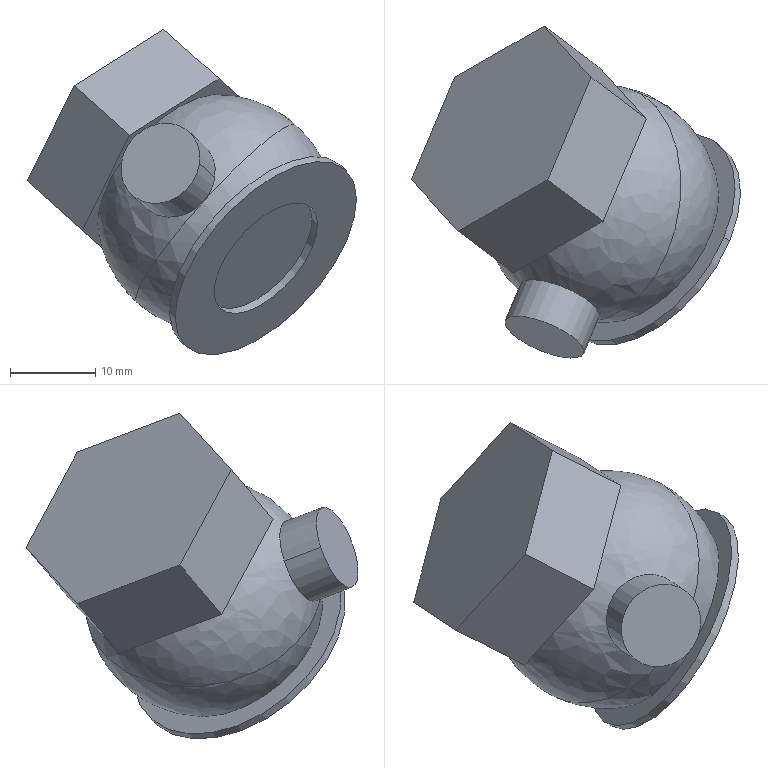Part | SolidWorks | features BaseBody 1 | 1 solid | 20 faces | box 38.707 x 39.047 x 38.307 mm | volume 14538 mm3 | plane 12 | cylinder 6 | spline 2 | commonest cylinder face diameters 10 x2 16 x2 28 x2
STEP:
#1=CARTESIAN_POINT('',(216.279,9.902,222.054));
#2=VERTEX_POINT('',#1);
#3=CARTESIAN_POINT('',(199.227,4.572,207.604));
#4=VERTEX_POINT('',#3);
#5=CARTESIAN_POINT('',(216.279,9.902,222.054));
#6=CARTESIAN_POINT('',(216.411,10.539,221.663));
#7=CARTESIAN_POINT('',(216.486,11.148,221.232));
#8=CARTESIAN_POINT('',(216.515,12.022,220.527));
#9=CARTESIAN_POINT('',(216.511,12.306,220.283));
#10=CARTESIAN_POINT('',(216.474,12.862,219.774));
#11=CARTESIAN_POINT('',(216.441,13.133,219.508));
#12=CARTESIAN_POINT('',(216.302,13.909,218.699));
#13=CARTESIAN_POINT('',(216.155,14.381,218.138));
#14=CARTESIAN_POINT('',(215.854,15.022,217.262));
#15=CARTESIAN_POINT('',(215.739,15.226,216.964));
#16=CARTESIAN_POINT('',(215.484,15.606,216.361));
#17=CARTESIAN_POINT('',(215.345,15.781,216.058));
#18=CARTESIAN_POINT('',(214.894,16.264,215.149));
#19=CARTESIAN_POINT('',(214.547,16.529,214.541));
#20=CARTESIAN_POINT('',(213.958,16.84,213.624));
#21=CARTESIAN_POINT('',(213.75,16.928,213.318));
#22=CARTESIAN_POINT('',(213.319,17.072,212.718));
#23=CARTESIAN_POINT('',(212.872,17.184,212.128));
#24=CARTESIAN_POINT('',(212.393,17.233,211.554));
#25=CARTESIAN_POINT('',(211.897,17.249,210.989));
#26=CARTESIAN_POINT('',(211.64,17.242,210.71));
#27=CARTESIAN_POINT('',(210.853,17.17,209.897));
#28=CARTESIAN_POINT('',(210.312,17.058,209.39));
#29=CARTESIAN_POINT('',(209.479,16.798,208.683));
#30=CARTESIAN_POINT('',(209.197,16.696,208.456));
#31=CARTESIAN_POINT('',(208.625,16.459,208.02));
#32=CARTESIAN_POINT('',(208.337,16.326,207.813));
#33=CARTESIAN_POINT('',(207.479,15.885,207.231));
#34=CARTESIAN_POINT('',(206.909,15.537,206.892));
#35=CARTESIAN_POINT('',(206.06,14.933,206.458));
#36=CARTESIAN_POINT('',(205.776,14.717,206.325));
#37=CARTESIAN_POINT('',(205.221,14.264,206.09));
#38=CARTESIAN_POINT('',(204.948,14.027,205.987));
#39=CARTESIAN_POINT('',(204.147,13.287,205.72));
#40=CARTESIAN_POINT('',(203.633,12.754,205.599));
#41=CARTESIAN_POINT('',(202.651,11.606,205.476));
#42=CARTESIAN_POINT('',(202.194,11.005,205.475));
#43=CARTESIAN_POINT('',(201.563,10.068,205.565));
#44=CARTESIAN_POINT('',(201.361,9.748,205.61));
#45=CARTESIAN_POINT('',(200.982,9.108,205.729));
#46=CARTESIAN_POINT('',(200.804,8.786,205.803));
#47=CARTESIAN_POINT('',(200.306,7.815,206.067));
#48=CARTESIAN_POINT('',(200.018,7.161,206.3));
#49=CARTESIAN_POINT('',(199.54,5.844,206.88));
#50=CARTESIAN_POINT('',(199.357,5.2,207.218));
#51=CARTESIAN_POINT('',(199.227,4.572,207.604));
#52=B_SPLINE_CURVE_WITH_KNOTS('',3,(#5,#6,#7,#8,#9,#10,#11,#12,#13,#14,#15,#16,#17,#18,#19,#20,#21,#22,#23,#24,#25,#26,#27,#28,#29,#30,#31,#32,#33,#34,#35,#36,#37,#38,#39,#40,#41,#42,#43,#44,#45,#46,#47,#48,#49,#50,#51),.UNSPECIFIED.,.F.,.F.,(4,2,2,2,2,2,2,2,2,1,2,2,2,2,2,2,2,2,2,2,2,2,2,4),(0.,0.002245,0.003367,0.004489,0.006734,0.007856,0.008978,0.01122,0.01235,0.01347,0.01459,0.01571,0.01796,0.01908,0.0202,0.02245,0.02357,0.02469,0.02694,0.02918,0.0303,0.03142,0.03367,0.03591),.UNSPECIFIED.);
#53=EDGE_CURVE('',#2,#4,#52,.T.);
#54=ORIENTED_EDGE('',*,*,#53,.T.);
#55=CARTESIAN_POINT('',(199.227,4.572,207.604));
#56=CARTESIAN_POINT('',(199.162,4.258,207.796));
#57=CARTESIAN_POINT('',(199.11,3.947,208.001));
#58=CARTESIAN_POINT('',(199.035,3.334,208.434));
#59=CARTESIAN_POINT('',(199.011,3.031,208.663));
#60=CARTESIAN_POINT('',(198.982,2.152,209.372));
#61=CARTESIAN_POINT('',(199.019,1.602,209.877));
#62=CARTESIAN_POINT('',(199.158,0.8279,210.684));
#63=CARTESIAN_POINT('',(199.219,0.5776,210.962));
#64=CARTESIAN_POINT('',(199.367,0.1001,211.53));
#65=CARTESIAN_POINT('',(199.455,-0.1256,211.818));
#66=CARTESIAN_POINT('',(199.756,-0.765,212.692));
#67=CARTESIAN_POINT('',(200.008,-1.141,213.289));
#68=CARTESIAN_POINT('',(200.463,-1.629,214.206));
#69=CARTESIAN_POINT('',(200.628,-1.777,214.514));
#70=CARTESIAN_POINT('',(200.976,-2.043,215.125));
#71=CARTESIAN_POINT('',(201.345,-2.278,215.733));
#72=CARTESIAN_POINT('',(201.755,-2.452,216.335));
#73=CARTESIAN_POINT('',(202.186,-2.596,216.935));
#74=CARTESIAN_POINT('',(202.412,-2.653,217.235));
#75=CARTESIAN_POINT('',(203.114,-2.774,218.116));
#76=CARTESIAN_POINT('',(203.608,-2.79,218.679));
#77=CARTESIAN_POINT('',(204.388,-2.719,219.485));
#78=CARTESIAN_POINT('',(204.655,-2.679,219.748));
#79=CARTESIAN_POINT('',(205.201,-2.567,220.26));
#80=CARTESIAN_POINT('',(205.479,-2.494,220.507));
#81=CARTESIAN_POINT('',(206.314,-2.233,221.216));
#82=CARTESIAN_POINT('',(206.88,-1.999,221.646));
#83=CARTESIAN_POINT('',(207.74,-1.558,222.23));
#84=CARTESIAN_POINT('',(208.031,-1.394,222.415));
#85=CARTESIAN_POINT('',(208.604,-1.043,222.756));
#86=CARTESIAN_POINT('',(208.888,-0.8549,222.913));
#87=CARTESIAN_POINT('',(209.733,-0.2537,223.344));
#88=CARTESIAN_POINT('',(210.285,0.1958,223.579));
#89=CARTESIAN_POINT('',(211.369,1.196,223.939));
#90=CARTESIAN_POINT('',(211.881,1.73,224.058));
#91=CARTESIAN_POINT('',(212.609,2.581,224.149));
#92=CARTESIAN_POINT('',(212.844,2.873,224.165));
#93=CARTESIAN_POINT('',(213.301,3.473,224.166));
#94=CARTESIAN_POINT('',(213.523,3.782,224.151));
#95=CARTESIAN_POINT('',(214.152,4.716,224.062));
#96=CARTESIAN_POINT('',(214.528,5.352,223.945));
#97=CARTESIAN_POINT('',(215.029,6.325,223.681));
#98=CARTESIAN_POINT('',(215.186,6.654,223.578));
#99=CARTESIAN_POINT('',(215.476,7.314,223.343));
#100=CARTESIAN_POINT('',(215.607,7.642,223.212));
#101=CARTESIAN_POINT('',(215.962,8.62,222.782));
#102=CARTESIAN_POINT('',(216.148,9.265,222.444));
#103=CARTESIAN_POINT('',(216.279,9.902,222.054));
#104=B_SPLINE_CURVE_WITH_KNOTS('',3,(#55,#56,#57,#58,#59,#60,#61,#62,#63,#64,#65,#66,#67,#68,#69,#70,#71,#72,#73,#74,#75,#76,#77,#78,#79,#80,#81,#82,#83,#84,#85,#86,#87,#88,#89,#90,#91,#92,#93,#94,#95,#96,#97,#98,#99,#100,#101,#102,#103),.UNSPECIFIED.,.F.,.F.,(4,2,2,2,2,2,2,2,1,2,2,2,2,2,2,2,2,2,2,2,2,2,2,2,4),(0.03591,0.03704,0.03816,0.0404,0.04153,0.04265,0.04489,0.04601,0.04714,0.04826,0.04938,0.05163,0.05275,0.05387,0.05612,0.05724,0.05836,0.0606,0.06285,0.06397,0.06509,0.06734,0.06846,0.06958,0.07183),.UNSPECIFIED.);
#105=EDGE_CURVE('',#4,#2,#104,.T.);
#106=ORIENTED_EDGE('',*,*,#105,.T.);
#107=EDGE_LOOP('',(#54,#106));
#108=FACE_BOUND('',#107,.T.);
#109=CARTESIAN_POINT('',(193.208,11.168,209.084));
#110=VERTEX_POINT('',#109);
#111=CARTESIAN_POINT('',(201.036,-2.678,220.875));
#112=VERTEX_POINT('',#111);
#113=CARTESIAN_POINT('',(202.575,11.168,219.49));
#114=DIRECTION('',(-0.7351,0.1479,0.6617));
#115=DIRECTION('',(-0.669,0.,-0.7432));
#116=AXIS2_PLACEMENT_3D('',#113,#114,#115);
#117=CIRCLE('',#116,14.);
#118=EDGE_CURVE('',#110,#112,#117,.T.);
#119=ORIENTED_EDGE('',*,*,#118,.F.);
#120=CARTESIAN_POINT('',(211.941,11.168,229.895));
#121=VERTEX_POINT('',#120);
#122=CARTESIAN_POINT('',(202.575,11.168,219.49));
#123=DIRECTION('',(0.7351,-0.1479,-0.6617));
#124=DIRECTION('',(-0.669,0.,-0.7432));
#125=AXIS2_PLACEMENT_3D('',#122,#123,#124);
#126=CIRCLE('',#125,14.);
#127=EDGE_CURVE('',#110,#121,#126,.T.);
#128=ORIENTED_EDGE('',*,*,#127,.T.);
#129=CARTESIAN_POINT('',(202.575,11.168,219.49));
#130=DIRECTION('',(-0.7351,0.1479,0.6617));
#131=DIRECTION('',(-0.669,0.,-0.7432));
#132=AXIS2_PLACEMENT_3D('',#129,#130,#131);
#133=CIRCLE('',#132,14.);
#134=EDGE_CURVE('',#112,#121,#133,.T.);
#135=ORIENTED_EDGE('',*,*,#134,.F.);
#136=EDGE_LOOP('',(#119,#128,#135));
#137=FACE_OUTER_BOUND('',#136,.T.);
#138=CARTESIAN_POINT('',(193.208,11.168,209.084));
#139=CARTESIAN_POINT('',(193.208,11.168,209.084));
#140=CARTESIAN_POINT('',(193.208,11.168,209.084));
#141=CARTESIAN_POINT('',(193.208,11.168,209.084));
#142=CARTESIAN_POINT('',(193.208,11.168,209.084));
#143=CARTESIAN_POINT('',(193.208,11.168,209.084));
#144=CARTESIAN_POINT('',(193.208,11.168,209.084));
#145=CARTESIAN_POINT('',(196.286,38.861,206.314));
#146=CARTESIAN_POINT('',(208.343,36.435,195.461));
#147=CARTESIAN_POINT('',(215.593,23.249,188.935));
#148=CARTESIAN_POINT('',(213.79,7.028,190.558));
#149=CARTESIAN_POINT('',(211.987,-9.194,192.18));
#150=CARTESIAN_POINT('',(202.187,-18.949,201.002));
#151=CARTESIAN_POINT('',(190.131,-16.524,211.855));
#152=CARTESIAN_POINT('',(215.019,38.861,227.125));
#153=CARTESIAN_POINT('',(227.075,36.435,216.272));
#154=CARTESIAN_POINT('',(234.326,23.249,209.746));
#155=CARTESIAN_POINT('',(232.523,7.028,211.368));
#156=CARTESIAN_POINT('',(230.72,-9.194,212.991));
#157=CARTESIAN_POINT('',(220.92,-18.949,221.813));
#158=CARTESIAN_POINT('',(208.863,-16.524,232.665));
#159=CARTESIAN_POINT('',(211.941,11.168,229.895));
#160=CARTESIAN_POINT('',(211.941,11.168,229.895));
#161=CARTESIAN_POINT('',(211.941,11.168,229.895));
#162=CARTESIAN_POINT('',(211.941,11.168,229.895));
#163=CARTESIAN_POINT('',(211.941,11.168,229.895));
#164=CARTESIAN_POINT('',(211.941,11.168,229.895));
#165=CARTESIAN_POINT('',(211.941,11.168,229.895));
#166=(BOUNDED_SURFACE()B_SPLINE_SURFACE(3,3,((#138,#139,#140,#141,#142,#143,#144),(#145,#146,#147,#148,#149,#150,#151),(#152,#153,#154,#155,#156,#157,#158),(#159,#160,#161,#162,#163,#164,#165)),.UNSPECIFIED.,.F.,.F.,.F.)B_SPLINE_SURFACE_WITH_KNOTS((4,4),(4,3,4),(0.,1.),(0.,0.5,1.),.UNSPECIFIED.)GEOMETRIC_REPRESENTATION_ITEM()RATIONAL_B_SPLINE_SURFACE(((1.,0.8047,0.8047,1.,0.8047,0.8047,1.),(0.3333,0.2682,0.2682,0.3333,0.2682,0.2682,0.3333),(0.3333,0.2682,0.2682,0.3333,0.2682,0.2682,0.3333),(1.,0.8047,0.8047,1.,0.8047,0.8047,1.)))REPRESENTATION_ITEM('')SURFACE());
#167=ADVANCED_FACE('',(#108,#137),#166,.T.);
#168=CARTESIAN_POINT('',(193.188,1.713,223.788));
#169=VERTEX_POINT('',#168);
#170=CARTESIAN_POINT('',(202.41,-2.154,223.788));
#171=VERTEX_POINT('',#170);
#172=CARTESIAN_POINT('',(197.799,-0.2209,223.788));
#173=DIRECTION('',(0.3652,0.871,-0.3287));
#174=DIRECTION('',(0.9222,-0.3867,0.));
#175=AXIS2_PLACEMENT_3D('',#172,#173,#174);
#176=CIRCLE('',#175,5.);
#177=EDGE_CURVE('',#169,#171,#176,.T.);
#178=ORIENTED_EDGE('',*,*,#177,.F.);
#179=CARTESIAN_POINT('',(191.39,-2.576,225.407));
#180=VERTEX_POINT('',#179);
#181=CARTESIAN_POINT('',(193.188,1.713,223.788));
#182=DIRECTION('',(-0.3652,-0.871,0.3287));
#183=VECTOR('',#182,1000.);
#184=LINE('',#181,#183);
#185=EDGE_CURVE('',#169,#180,#184,.T.);
#186=ORIENTED_EDGE('',*,*,#185,.T.);
#187=CARTESIAN_POINT('',(200.612,-6.442,225.407));
#188=VERTEX_POINT('',#187);
#189=CARTESIAN_POINT('',(196.001,-4.509,225.407));
#190=DIRECTION('',(0.3652,0.871,-0.3287));
#191=DIRECTION('',(0.9222,-0.3867,0.));
#192=AXIS2_PLACEMENT_3D('',#189,#190,#191);
#193=CIRCLE('',#192,5.);
#194=EDGE_CURVE('',#180,#188,#193,.T.);
#195=ORIENTED_EDGE('',*,*,#194,.T.);
#196=CARTESIAN_POINT('',(202.41,-2.154,223.788));
#197=DIRECTION('',(-0.3652,-0.871,0.3287));
#198=VECTOR('',#197,1000.);
#199=LINE('',#196,#198);
#200=EDGE_CURVE('',#171,#188,#199,.T.);
#201=ORIENTED_EDGE('',*,*,#200,.F.);
#202=EDGE_LOOP('',(#178,#186,#195,#201));
#203=FACE_OUTER_BOUND('',#202,.T.);
#204=CARTESIAN_POINT('',(197.799,-0.2209,223.788));
#205=DIRECTION('',(-0.3652,-0.871,0.3287));
#206=DIRECTION('',(0.9222,-0.3867,0.));
#207=AXIS2_PLACEMENT_3D('',#204,#205,#206);
#208=CYLINDRICAL_SURFACE('',#207,5.);
#209=ADVANCED_FACE('',(#203),#208,.T.);
#210=CARTESIAN_POINT('',(198.387,7.238,204.423));
#211=VERTEX_POINT('',#210);
#212=CARTESIAN_POINT('',(217.12,7.238,225.233));
#213=VERTEX_POINT('',#212);
#214=CARTESIAN_POINT('',(207.753,7.238,214.828));
#215=DIRECTION('',(0.6473,-0.4913,-0.5827));
#216=DIRECTION('',(-0.669,0.,-0.7432));
#217=AXIS2_PLACEMENT_3D('',#214,#215,#216);
#218=CIRCLE('',#217,14.);
#219=EDGE_CURVE('',#211,#213,#218,.T.);
#220=ORIENTED_EDGE('',*,*,#219,.T.);
#221=CARTESIAN_POINT('',(217.767,6.746,224.651));
#222=VERTEX_POINT('',#221);
#223=CARTESIAN_POINT('',(217.12,7.238,225.233));
#224=DIRECTION('',(0.6473,-0.4913,-0.5827));
#225=VECTOR('',#224,1000.);
#226=LINE('',#223,#225);
#227=EDGE_CURVE('',#213,#222,#226,.T.);
#228=ORIENTED_EDGE('',*,*,#227,.T.);
#229=CARTESIAN_POINT('',(199.034,6.746,203.84));
#230=VERTEX_POINT('',#229);
#231=CARTESIAN_POINT('',(208.401,6.746,214.245));
#232=DIRECTION('',(-0.6473,0.4913,0.5827));
#233=DIRECTION('',(-0.669,0.,-0.7432));
#234=AXIS2_PLACEMENT_3D('',#231,#232,#233);
#235=CIRCLE('',#234,14.);
#236=EDGE_CURVE('',#222,#230,#235,.T.);
#237=ORIENTED_EDGE('',*,*,#236,.T.);
#238=CARTESIAN_POINT('',(198.387,7.238,204.423));
#239=DIRECTION('',(0.6473,-0.4913,-0.5827));
#240=VECTOR('',#239,1000.);
#241=LINE('',#238,#240);
#242=EDGE_CURVE('',#211,#230,#241,.T.);
#243=ORIENTED_EDGE('',*,*,#242,.F.);
#244=EDGE_LOOP('',(#220,#228,#237,#243));
#245=FACE_OUTER_BOUND('',#244,.T.);
#246=CARTESIAN_POINT('',(207.753,7.238,214.828));
#247=DIRECTION('',(0.6473,-0.4913,-0.5827));
#248=DIRECTION('',(-0.669,0.,-0.7432));
#249=AXIS2_PLACEMENT_3D('',#246,#247,#248);
#250=CYLINDRICAL_SURFACE('',#249,14.);
#251=ADVANCED_FACE('',(#245),#250,.T.);
#252=CARTESIAN_POINT('',(203.048,6.746,208.299));
#253=VERTEX_POINT('',#252);
#254=CARTESIAN_POINT('',(213.753,6.746,220.191));
#255=VERTEX_POINT('',#254);
#256=CARTESIAN_POINT('',(208.401,6.746,214.245));
#257=DIRECTION('',(-0.6473,0.4913,0.5827));
#258=DIRECTION('',(0.669,0.,0.7432));
#259=AXIS2_PLACEMENT_3D('',#256,#257,#258);
#260=CIRCLE('',#259,8.);
#261=EDGE_CURVE('',#253,#255,#260,.T.);
#262=ORIENTED_EDGE('',*,*,#261,.F.);
#263=CARTESIAN_POINT('',(202.401,7.238,208.882));
#264=VERTEX_POINT('',#263);
#265=CARTESIAN_POINT('',(203.048,6.746,208.299));
#266=DIRECTION('',(-0.6473,0.4913,0.5827));
#267=VECTOR('',#266,1000.);
#268=LINE('',#265,#267);
#269=EDGE_CURVE('',#253,#264,#268,.T.);
#270=ORIENTED_EDGE('',*,*,#269,.T.);
#271=CARTESIAN_POINT('',(213.106,7.238,220.774));
#272=VERTEX_POINT('',#271);
#273=CARTESIAN_POINT('',(207.753,7.238,214.828));
#274=DIRECTION('',(0.6473,-0.4913,-0.5827));
#275=DIRECTION('',(0.669,0.,0.7432));
#276=AXIS2_PLACEMENT_3D('',#273,#274,#275);
#277=CIRCLE('',#276,8.);
#278=EDGE_CURVE('',#272,#264,#277,.T.);
#279=ORIENTED_EDGE('',*,*,#278,.F.);
#280=CARTESIAN_POINT('',(213.753,6.746,220.191));
#281=DIRECTION('',(-0.6473,0.4913,0.5827));
#282=VECTOR('',#281,1000.);
#283=LINE('',#280,#282);
#284=EDGE_CURVE('',#255,#272,#283,.T.);
#285=ORIENTED_EDGE('',*,*,#284,.F.);
#286=EDGE_LOOP('',(#262,#270,#279,#285));
#287=FACE_OUTER_BOUND('',#286,.T.);
#288=CARTESIAN_POINT('',(208.401,6.746,214.245));
#289=DIRECTION('',(-0.6473,0.4913,0.5827));
#290=DIRECTION('',(0.669,0.,0.7432));
#291=AXIS2_PLACEMENT_3D('',#288,#289,#290);
#292=CYLINDRICAL_SURFACE('',#291,8.);
#293=ADVANCED_FACE('',(#287),#292,.F.);
#294=ORIENTED_EDGE('',*,*,#127,.F.);
#295=ORIENTED_EDGE('',*,*,#118,.T.);
#296=CARTESIAN_POINT('',(197.799,-0.2209,223.788));
#297=DIRECTION('',(0.3652,0.871,-0.3287));
#298=DIRECTION('',(0.9222,-0.3867,0.));
#299=AXIS2_PLACEMENT_3D('',#296,#297,#298);
#300=CIRCLE('',#299,5.);
#301=EDGE_CURVE('',#112,#169,#300,.T.);
#302=ORIENTED_EDGE('',*,*,#301,.T.);
#303=ORIENTED_EDGE('',*,*,#177,.T.);
#304=CARTESIAN_POINT('',(197.799,-0.2209,223.788));
#305=DIRECTION('',(0.3652,0.871,-0.3287));
#306=DIRECTION('',(0.9222,-0.3867,0.));
#307=AXIS2_PLACEMENT_3D('',#304,#305,#306);
#308=CIRCLE('',#307,5.);
#309=EDGE_CURVE('',#171,#112,#308,.T.);
#310=ORIENTED_EDGE('',*,*,#309,.T.);
#311=ORIENTED_EDGE('',*,*,#134,.T.);
#312=EDGE_LOOP('',(#294,#295,#302,#303,#310,#311));
#313=FACE_OUTER_BOUND('',#312,.T.);
#314=CARTESIAN_POINT('',(188.87,12.435,216.926));
#315=VERTEX_POINT('',#314);
#316=CARTESIAN_POINT('',(205.923,17.769,231.373));
#317=VERTEX_POINT('',#316);
#318=CARTESIAN_POINT('',(188.87,12.435,216.926));
#319=CARTESIAN_POINT('',(189.002,13.072,216.535));
#320=CARTESIAN_POINT('',(189.187,13.716,216.198));
#321=CARTESIAN_POINT('',(189.541,14.691,215.769));
#322=CARTESIAN_POINT('',(189.672,15.018,215.638));
#323=CARTESIAN_POINT('',(189.959,15.675,215.404));
#324=CARTESIAN_POINT('',(190.117,16.005,215.3));
#325=CARTESIAN_POINT('',(190.619,16.982,215.035));
#326=CARTESIAN_POINT('',(190.996,17.618,214.918));
#327=CARTESIAN_POINT('',(191.623,18.549,214.829));
#328=CARTESIAN_POINT('',(191.843,18.857,214.814));
#329=CARTESIAN_POINT('',(192.301,19.46,214.814));
#330=CARTESIAN_POINT('',(192.537,19.752,214.83));
#331=CARTESIAN_POINT('',(193.265,20.604,214.921));
#332=CARTESIAN_POINT('',(193.777,21.137,215.04));
#333=CARTESIAN_POINT('',(194.586,21.884,215.308));
#334=CARTESIAN_POINT('',(194.862,22.124,215.412));
#335=CARTESIAN_POINT('',(195.416,22.576,215.647));
#336=CARTESIAN_POINT('',(195.974,23.002,215.908));
#337=CARTESIAN_POINT('',(196.541,23.377,216.221));
#338=CARTESIAN_POINT('',(197.113,23.728,216.561));
#339=CARTESIAN_POINT('',(197.403,23.891,216.745));
#340=CARTESIAN_POINT('',(198.266,24.335,217.331));
#341=CARTESIAN_POINT('',(198.832,24.569,217.762));
#342=CARTESIAN_POINT('',(199.666,24.83,218.468));
#343=CARTESIAN_POINT('',(199.942,24.902,218.714));
#344=CARTESIAN_POINT('',(200.488,25.015,219.225));
#345=CARTESIAN_POINT('',(200.757,25.055,219.49));
#346=CARTESIAN_POINT('',(201.539,25.127,220.298));
#347=CARTESIAN_POINT('',(202.033,25.111,220.86));
#348=CARTESIAN_POINT('',(202.732,24.991,221.738));
#349=CARTESIAN_POINT('',(202.959,24.934,222.038));
#350=CARTESIAN_POINT('',(203.391,24.79,222.64));
#351=CARTESIAN_POINT('',(203.597,24.703,222.942));
#352=CARTESIAN_POINT('',(204.181,24.396,223.85));
#353=CARTESIAN_POINT('',(204.529,24.132,224.459));
#354=CARTESIAN_POINT('',(205.139,23.481,225.686));
#355=CARTESIAN_POINT('',(205.392,23.104,226.285));
#356=CARTESIAN_POINT('',(205.693,22.465,227.157));
#357=CARTESIAN_POINT('',(205.781,22.24,227.444));
#358=CARTESIAN_POINT('',(205.929,21.765,228.01));
#359=CARTESIAN_POINT('',(205.99,21.514,228.29));
#360=CARTESIAN_POINT('',(206.13,20.738,229.1));
#361=CARTESIAN_POINT('',(206.167,20.187,229.605));
#362=CARTESIAN_POINT('',(206.13,19.02,230.548));
#363=CARTESIAN_POINT('',(206.053,18.398,230.987));
#364=CARTESIAN_POINT('',(205.923,17.769,231.373));
#365=B_SPLINE_CURVE_WITH_KNOTS('',3,(#318,#319,#320,#321,#322,#323,#324,#325,#326,#327,#328,#329,#330,#331,#332,#333,#334,#335,#336,#337,#338,#339,#340,#341,#342,#343,#344,#345,#346,#347,#348,#349,#350,#351,#352,#353,#354,#355,#356,#357,#358,#359,#360,#361,#362,#363,#364),.UNSPECIFIED.,.F.,.F.,(4,2,2,2,2,2,2,2,2,1,2,2,2,2,2,2,2,2,2,2,2,2,2,4),(0.,0.002245,0.003367,0.004489,0.006734,0.007856,0.008978,0.01122,0.01235,0.01347,0.01459,0.01571,0.01796,0.01908,0.0202,0.02245,0.02357,0.02469,0.02694,0.02918,0.0303,0.03142,0.03367,0.03591),.UNSPECIFIED.);
#366=EDGE_CURVE('',#315,#317,#365,.T.);
#367=ORIENTED_EDGE('',*,*,#366,.T.);
#368=CARTESIAN_POINT('',(205.923,17.769,231.373));
#369=CARTESIAN_POINT('',(205.793,17.139,231.76));
#370=CARTESIAN_POINT('',(205.61,16.497,232.098));
#371=CARTESIAN_POINT('',(205.254,15.514,232.531));
#372=CARTESIAN_POINT('',(205.121,15.182,232.663));
#373=CARTESIAN_POINT('',(204.834,14.526,232.897));
#374=CARTESIAN_POINT('',(204.523,13.874,233.102));
#375=CARTESIAN_POINT('',(204.167,13.23,233.25));
#376=CARTESIAN_POINT('',(203.788,12.589,233.37));
#377=CARTESIAN_POINT('',(203.586,12.269,233.415));
#378=CARTESIAN_POINT('',(202.957,11.334,233.504));
#379=CARTESIAN_POINT('',(202.504,10.739,233.503));
#380=CARTESIAN_POINT('',(201.532,9.601,233.383));
#381=CARTESIAN_POINT('',(201.009,9.056,233.261));
#382=CARTESIAN_POINT('',(199.939,8.067,232.906));
#383=CARTESIAN_POINT('',(199.388,7.617,232.673));
#384=CARTESIAN_POINT('',(198.537,7.01,232.239));
#385=CARTESIAN_POINT('',(198.248,6.82,232.08));
#386=CARTESIAN_POINT('',(197.676,6.469,231.74));
#387=CARTESIAN_POINT('',(197.105,6.147,231.376));
#388=CARTESIAN_POINT('',(196.536,5.883,230.967));
#389=CARTESIAN_POINT('',(195.968,5.647,230.536));
#390=CARTESIAN_POINT('',(195.684,5.543,230.307));
#391=CARTESIAN_POINT('',(194.841,5.279,229.594));
#392=CARTESIAN_POINT('',(194.301,5.168,229.087));
#393=CARTESIAN_POINT('',(193.521,5.096,228.281));
#394=CARTESIAN_POINT('',(193.266,5.088,228.005));
#395=CARTESIAN_POINT('',(192.767,5.103,227.438));
#396=CARTESIAN_POINT('',(192.524,5.128,227.147));
#397=CARTESIAN_POINT('',(191.826,5.248,226.27));
#398=CARTESIAN_POINT('',(191.397,5.39,225.673));
#399=CARTESIAN_POINT('',(190.809,5.698,224.761));
#400=CARTESIAN_POINT('',(190.621,5.817,224.452));
#401=CARTESIAN_POINT('',(190.271,6.084,223.838));
#402=CARTESIAN_POINT('',(190.108,6.231,223.534));
#403=CARTESIAN_POINT('',(189.657,6.713,222.625));
#404=CARTESIAN_POINT('',(189.404,7.088,222.028));
#405=CARTESIAN_POINT('',(189.098,7.734,221.144));
#406=CARTESIAN_POINT('',(189.01,7.961,220.855));
#407=CARTESIAN_POINT('',(188.862,8.434,220.291));
#408=CARTESIAN_POINT('',(188.742,8.928,219.741));
#409=CARTESIAN_POINT('',(188.677,9.462,219.218));
#410=CARTESIAN_POINT('',(188.639,10.015,218.71));
#411=CARTESIAN_POINT('',(188.634,10.304,218.461));
#412=CARTESIAN_POINT('',(188.663,11.186,217.749));
#413=CARTESIAN_POINT('',(188.738,11.798,217.316));
#414=CARTESIAN_POINT('',(188.87,12.435,216.926));
#415=B_SPLINE_CURVE_WITH_KNOTS('',3,(#368,#369,#370,#371,#372,#373,#374,#375,#376,#377,#378,#379,#380,#381,#382,#383,#384,#385,#386,#387,#388,#389,#390,#391,#392,#393,#394,#395,#396,#397,#398,#399,#400,#401,#402,#403,#404,#405,#406,#407,#408,#409,#410,#411,#412,#413,#414),.UNSPECIFIED.,.F.,.F.,(4,2,2,1,2,2,2,2,2,2,1,2,2,2,2,2,2,2,2,2,2,1,2,2,4),(0.03591,0.03816,0.03928,0.0404,0.04153,0.04265,0.04489,0.04714,0.04938,0.0505,0.05163,0.05275,0.05387,0.05612,0.05724,0.05836,0.0606,0.06173,0.06285,0.06509,0.06622,0.06734,0.06846,0.06958,0.07183),.UNSPECIFIED.);
#416=EDGE_CURVE('',#317,#315,#415,.T.);
#417=ORIENTED_EDGE('',*,*,#416,.T.);
#418=EDGE_LOOP('',(#367,#417));
#419=FACE_BOUND('',#418,.T.);
#420=CARTESIAN_POINT('',(193.208,11.168,209.084));
#421=CARTESIAN_POINT('',(193.208,11.168,209.084));
#422=CARTESIAN_POINT('',(193.208,11.168,209.084));
#423=CARTESIAN_POINT('',(193.208,11.168,209.084));
#424=CARTESIAN_POINT('',(190.131,-16.524,211.855));
#425=CARTESIAN_POINT('',(148.967,-8.242,248.908));
#426=CARTESIAN_POINT('',(155.122,47.142,243.367));
#427=CARTESIAN_POINT('',(196.286,38.861,206.314));
#428=CARTESIAN_POINT('',(208.863,-16.524,232.665));
#429=CARTESIAN_POINT('',(167.7,-8.242,269.719));
#430=CARTESIAN_POINT('',(173.855,47.142,264.178));
#431=CARTESIAN_POINT('',(215.019,38.861,227.125));
#432=CARTESIAN_POINT('',(211.941,11.168,229.895));
#433=CARTESIAN_POINT('',(211.941,11.168,229.895));
#434=CARTESIAN_POINT('',(211.941,11.168,229.895));
#435=CARTESIAN_POINT('',(211.941,11.168,229.895));
#436=(BOUNDED_SURFACE()B_SPLINE_SURFACE(3,3,((#420,#421,#422,#423),(#424,#425,#426,#427),(#428,#429,#430,#431),(#432,#433,#434,#435)),.UNSPECIFIED.,.F.,.F.,.T.)B_SPLINE_SURFACE_WITH_KNOTS((4,4),(4,4),(0.,1.),(0.,1.),.UNSPECIFIED.)GEOMETRIC_REPRESENTATION_ITEM()RATIONAL_B_SPLINE_SURFACE(((1.,0.3333,0.3333,1.),(0.3333,0.1111,0.1111,0.3333),(0.3333,0.1111,0.1111,0.3333),(1.,0.3333,0.3333,1.)))REPRESENTATION_ITEM('')SURFACE());
#437=ADVANCED_FACE('',(#313,#419),#436,.T.);
#438=ORIENTED_EDGE('',*,*,#366,.F.);
#439=ORIENTED_EDGE('',*,*,#416,.F.);
#440=EDGE_LOOP('',(#438,#439));
#441=FACE_BOUND('',#440,.T.);
#442=CARTESIAN_POINT('',(202.456,27.168,219.596));
#443=VERTEX_POINT('',#442);
#444=CARTESIAN_POINT('',(207.954,21.133,230.793));
#445=VERTEX_POINT('',#444);
#446=CARTESIAN_POINT('',(202.456,27.168,219.596));
#447=DIRECTION('',(0.3968,-0.4355,0.808));
#448=VECTOR('',#447,1000.);
#449=LINE('',#446,#448);
#450=EDGE_CURVE('',#443,#445,#449,.T.);
#451=ORIENTED_EDGE('',*,*,#450,.T.);
#452=CARTESIAN_POINT('',(202.894,9.065,235.348));
#453=VERTEX_POINT('',#452);
#454=CARTESIAN_POINT('',(205.424,15.099,233.07));
#455=DIRECTION('',(-0.3652,-0.871,0.3287));
#456=VECTOR('',#455,1000.);
#457=LINE('',#454,#456);
#458=EDGE_CURVE('',#445,#453,#457,.T.);
#459=ORIENTED_EDGE('',*,*,#458,.T.);
#460=CARTESIAN_POINT('',(192.336,3.031,228.706));
#461=VERTEX_POINT('',#460);
#462=CARTESIAN_POINT('',(202.894,9.065,235.348));
#463=DIRECTION('',(-0.762,-0.4355,-0.4793));
#464=VECTOR('',#463,1000.);
#465=LINE('',#462,#464);
#466=EDGE_CURVE('',#453,#461,#465,.T.);
#467=ORIENTED_EDGE('',*,*,#466,.T.);
#468=CARTESIAN_POINT('',(186.838,9.065,217.51));
#469=VERTEX_POINT('',#468);
#470=CARTESIAN_POINT('',(192.336,3.031,228.706));
#471=DIRECTION('',(-0.3968,0.4355,-0.808));
#472=VECTOR('',#471,1000.);
#473=LINE('',#470,#472);
#474=EDGE_CURVE('',#461,#469,#473,.T.);
#475=ORIENTED_EDGE('',*,*,#474,.T.);
#476=CARTESIAN_POINT('',(191.898,21.133,212.955));
#477=VERTEX_POINT('',#476);
#478=CARTESIAN_POINT('',(189.368,15.099,215.232));
#479=DIRECTION('',(0.3652,0.871,-0.3287));
#480=VECTOR('',#479,1000.);
#481=LINE('',#478,#480);
#482=EDGE_CURVE('',#469,#477,#481,.T.);
#483=ORIENTED_EDGE('',*,*,#482,.T.);
#484=CARTESIAN_POINT('',(191.898,21.133,212.955));
#485=DIRECTION('',(0.762,0.4355,0.4793));
#486=VECTOR('',#485,1000.);
#487=LINE('',#484,#486);
#488=EDGE_CURVE('',#477,#443,#487,.T.);
#489=ORIENTED_EDGE('',*,*,#488,.T.);
#490=EDGE_LOOP('',(#451,#459,#467,#475,#483,#489));
#491=FACE_OUTER_BOUND('',#490,.T.);
#492=CARTESIAN_POINT('',(197.396,15.099,224.151));
#493=DIRECTION('',(0.6473,-0.4913,-0.5827));
#494=DIRECTION('',(-0.669,0.,-0.7432));
#495=AXIS2_PLACEMENT_3D('',#492,#493,#494);
#496=PLANE('',#495);
#497=ADVANCED_FACE('',(#441,#491),#496,.T.);
#498=ORIENTED_EDGE('',*,*,#53,.F.);
#499=ORIENTED_EDGE('',*,*,#105,.F.);
#500=EDGE_LOOP('',(#498,#499));
#501=FACE_BOUND('',#500,.T.);
#502=ORIENTED_EDGE('',*,*,#219,.F.);
#503=CARTESIAN_POINT('',(207.753,7.238,214.828));
#504=DIRECTION('',(0.6473,-0.4913,-0.5827));
#505=DIRECTION('',(-0.669,0.,-0.7432));
#506=AXIS2_PLACEMENT_3D('',#503,#504,#505);
#507=CIRCLE('',#506,14.);
#508=EDGE_CURVE('',#213,#211,#507,.T.);
#509=ORIENTED_EDGE('',*,*,#508,.F.);
#510=EDGE_LOOP('',(#502,#509));
#511=FACE_OUTER_BOUND('',#510,.T.);
#512=CARTESIAN_POINT('',(207.753,7.238,214.828));
#513=DIRECTION('',(0.6473,-0.4913,-0.5827));
#514=DIRECTION('',(-0.669,0.,-0.7432));
#515=AXIS2_PLACEMENT_3D('',#512,#513,#514);
#516=PLANE('',#515);
#517=ADVANCED_FACE('',(#501,#511),#516,.F.);
#518=ORIENTED_EDGE('',*,*,#458,.F.);
#519=CARTESIAN_POINT('',(201.481,26.047,236.62));
#520=VERTEX_POINT('',#519);
#521=CARTESIAN_POINT('',(207.954,21.133,230.793));
#522=DIRECTION('',(-0.6473,0.4913,0.5827));
#523=VECTOR('',#522,1000.);
#524=LINE('',#521,#523);
#525=EDGE_CURVE('',#445,#520,#524,.T.);
#526=ORIENTED_EDGE('',*,*,#525,.T.);
#527=CARTESIAN_POINT('',(196.421,13.978,241.175));
#528=VERTEX_POINT('',#527);
#529=CARTESIAN_POINT('',(201.481,26.047,236.62));
#530=DIRECTION('',(-0.3652,-0.871,0.3287));
#531=VECTOR('',#530,1000.);
#532=LINE('',#529,#531);
#533=EDGE_CURVE('',#520,#528,#532,.T.);
#534=ORIENTED_EDGE('',*,*,#533,.T.);
#535=CARTESIAN_POINT('',(196.421,13.978,241.175));
#536=DIRECTION('',(0.6473,-0.4913,-0.5827));
#537=VECTOR('',#536,1000.);
#538=LINE('',#535,#537);
#539=EDGE_CURVE('',#528,#453,#538,.T.);
#540=ORIENTED_EDGE('',*,*,#539,.T.);
#541=EDGE_LOOP('',(#518,#526,#534,#540));
#542=FACE_OUTER_BOUND('',#541,.T.);
#543=CARTESIAN_POINT('',(202.188,17.556,235.984));
#544=DIRECTION('',(0.669,0.,0.7432));
#545=DIRECTION('',(0.7432,0.,-0.669));
#546=AXIS2_PLACEMENT_3D('',#543,#544,#545);
#547=PLANE('',#546);
#548=ADVANCED_FACE('',(#542),#547,.T.);
#549=ORIENTED_EDGE('',*,*,#450,.F.);
#550=CARTESIAN_POINT('',(195.983,32.081,225.423));
#551=VERTEX_POINT('',#550);
#552=CARTESIAN_POINT('',(202.456,27.168,219.596));
#553=DIRECTION('',(-0.6473,0.4913,0.5827));
#554=VECTOR('',#553,1000.);
#555=LINE('',#552,#554);
#556=EDGE_CURVE('',#443,#551,#555,.T.);
#557=ORIENTED_EDGE('',*,*,#556,.T.);
#558=CARTESIAN_POINT('',(195.983,32.081,225.423));
#559=DIRECTION('',(0.3968,-0.4355,0.808));
#560=VECTOR('',#559,1000.);
#561=LINE('',#558,#560);
#562=EDGE_CURVE('',#551,#520,#561,.T.);
#563=ORIENTED_EDGE('',*,*,#562,.T.);
#564=ORIENTED_EDGE('',*,*,#525,.F.);
#565=EDGE_LOOP('',(#549,#557,#563,#564));
#566=FACE_OUTER_BOUND('',#565,.T.);
#567=CARTESIAN_POINT('',(201.969,26.607,228.108));
#568=DIRECTION('',(0.6508,0.7543,0.08694));
#569=DIRECTION('',(-0.7571,0.6532,0.));
#570=AXIS2_PLACEMENT_3D('',#567,#568,#569);
#571=PLANE('',#570);
#572=ADVANCED_FACE('',(#566),#571,.T.);
#573=ORIENTED_EDGE('',*,*,#488,.F.);
#574=CARTESIAN_POINT('',(185.424,26.047,218.782));
#575=VERTEX_POINT('',#574);
#576=CARTESIAN_POINT('',(191.898,21.133,212.955));
#577=DIRECTION('',(-0.6473,0.4913,0.5827));
#578=VECTOR('',#577,1000.);
#579=LINE('',#576,#578);
#580=EDGE_CURVE('',#477,#575,#579,.T.);
#581=ORIENTED_EDGE('',*,*,#580,.T.);
#582=CARTESIAN_POINT('',(185.424,26.047,218.782));
#583=DIRECTION('',(0.762,0.4355,0.4793));
#584=VECTOR('',#583,1000.);
#585=LINE('',#582,#584);
#586=EDGE_CURVE('',#575,#551,#585,.T.);
#587=ORIENTED_EDGE('',*,*,#586,.T.);
#588=ORIENTED_EDGE('',*,*,#556,.F.);
#589=EDGE_LOOP('',(#573,#581,#587,#588));
#590=FACE_OUTER_BOUND('',#589,.T.);
#591=CARTESIAN_POINT('',(193.94,26.607,219.189));
#592=DIRECTION('',(-0.01825,0.7543,-0.6563));
#593=DIRECTION('',(0.,0.6564,0.7544));
#594=AXIS2_PLACEMENT_3D('',#591,#592,#593);
#595=PLANE('',#594);
#596=ADVANCED_FACE('',(#590),#595,.T.);
#597=ORIENTED_EDGE('',*,*,#580,.F.);
#598=ORIENTED_EDGE('',*,*,#482,.F.);
#599=CARTESIAN_POINT('',(180.364,13.978,223.337));
#600=VERTEX_POINT('',#599);
#601=CARTESIAN_POINT('',(180.364,13.978,223.337));
#602=DIRECTION('',(0.6473,-0.4913,-0.5827));
#603=VECTOR('',#602,1000.);
#604=LINE('',#601,#603);
#605=EDGE_CURVE('',#600,#469,#604,.T.);
#606=ORIENTED_EDGE('',*,*,#605,.F.);
#607=CARTESIAN_POINT('',(185.424,26.047,218.782));
#608=DIRECTION('',(-0.3652,-0.871,0.3287));
#609=VECTOR('',#608,1000.);
#610=LINE('',#607,#609);
#611=EDGE_CURVE('',#575,#600,#610,.T.);
#612=ORIENTED_EDGE('',*,*,#611,.F.);
#613=EDGE_LOOP('',(#597,#598,#606,#612));
#614=FACE_OUTER_BOUND('',#613,.T.);
#615=CARTESIAN_POINT('',(186.131,17.556,218.146));
#616=DIRECTION('',(0.669,0.,0.7432));
#617=DIRECTION('',(0.7432,0.,-0.669));
#618=AXIS2_PLACEMENT_3D('',#615,#616,#617);
#619=PLANE('',#618);
#620=ADVANCED_FACE('',(#614),#619,.F.);
#621=ORIENTED_EDGE('',*,*,#605,.T.);
#622=ORIENTED_EDGE('',*,*,#474,.F.);
#623=CARTESIAN_POINT('',(185.862,7.944,234.533));
#624=VERTEX_POINT('',#623);
#625=CARTESIAN_POINT('',(185.862,7.944,234.533));
#626=DIRECTION('',(0.6473,-0.4913,-0.5827));
#627=VECTOR('',#626,1000.);
#628=LINE('',#625,#627);
#629=EDGE_CURVE('',#624,#461,#628,.T.);
#630=ORIENTED_EDGE('',*,*,#629,.F.);
#631=CARTESIAN_POINT('',(180.364,13.978,223.337));
#632=DIRECTION('',(0.3968,-0.4355,0.808));
#633=VECTOR('',#632,1000.);
#634=LINE('',#631,#633);
#635=EDGE_CURVE('',#600,#624,#634,.T.);
#636=ORIENTED_EDGE('',*,*,#635,.F.);
#637=EDGE_LOOP('',(#621,#622,#630,#636));
#638=FACE_OUTER_BOUND('',#637,.T.);
#639=CARTESIAN_POINT('',(186.35,8.505,226.021));
#640=DIRECTION('',(0.6508,0.7543,0.08694));
#641=DIRECTION('',(-0.7571,0.6532,0.));
#642=AXIS2_PLACEMENT_3D('',#639,#640,#641);
#643=PLANE('',#642);
#644=ADVANCED_FACE('',(#638),#643,.F.);
#645=ORIENTED_EDGE('',*,*,#629,.T.);
#646=ORIENTED_EDGE('',*,*,#466,.F.);
#647=ORIENTED_EDGE('',*,*,#539,.F.);
#648=CARTESIAN_POINT('',(185.862,7.944,234.533));
#649=DIRECTION('',(0.762,0.4355,0.4793));
#650=VECTOR('',#649,1000.);
#651=LINE('',#648,#650);
#652=EDGE_CURVE('',#624,#528,#651,.T.);
#653=ORIENTED_EDGE('',*,*,#652,.F.);
#654=EDGE_LOOP('',(#645,#646,#647,#653));
#655=FACE_OUTER_BOUND('',#654,.T.);
#656=CARTESIAN_POINT('',(194.378,8.505,234.94));
#657=DIRECTION('',(-0.01825,0.7543,-0.6563));
#658=DIRECTION('',(0.,0.6564,0.7544));
#659=AXIS2_PLACEMENT_3D('',#656,#657,#658);
#660=PLANE('',#659);
#661=ADVANCED_FACE('',(#655),#660,.F.);
#662=ORIENTED_EDGE('',*,*,#185,.F.);
#663=ORIENTED_EDGE('',*,*,#301,.F.);
#664=ORIENTED_EDGE('',*,*,#309,.F.);
#665=ORIENTED_EDGE('',*,*,#200,.T.);
#666=CARTESIAN_POINT('',(196.001,-4.509,225.407));
#667=DIRECTION('',(0.3652,0.871,-0.3287));
#668=DIRECTION('',(0.9222,-0.3867,0.));
#669=AXIS2_PLACEMENT_3D('',#666,#667,#668);
#670=CIRCLE('',#669,5.);
#671=EDGE_CURVE('',#188,#180,#670,.T.);
#672=ORIENTED_EDGE('',*,*,#671,.T.);
#673=EDGE_LOOP('',(#662,#663,#664,#665,#672));
#674=FACE_OUTER_BOUND('',#673,.T.);
#675=CARTESIAN_POINT('',(197.799,-0.2209,223.788));
#676=DIRECTION('',(-0.3652,-0.871,0.3287));
#677=DIRECTION('',(0.9222,-0.3867,0.));
#678=AXIS2_PLACEMENT_3D('',#675,#676,#677);
#679=CYLINDRICAL_SURFACE('',#678,5.);
#680=ADVANCED_FACE('',(#674),#679,.T.);
#681=ORIENTED_EDGE('',*,*,#227,.F.);
#682=ORIENTED_EDGE('',*,*,#508,.T.);
#683=ORIENTED_EDGE('',*,*,#242,.T.);
#684=CARTESIAN_POINT('',(208.401,6.746,214.245));
#685=DIRECTION('',(-0.6473,0.4913,0.5827));
#686=DIRECTION('',(-0.669,0.,-0.7432));
#687=AXIS2_PLACEMENT_3D('',#684,#685,#686);
#688=CIRCLE('',#687,14.);
#689=EDGE_CURVE('',#230,#222,#688,.T.);
#690=ORIENTED_EDGE('',*,*,#689,.T.);
#691=EDGE_LOOP('',(#681,#682,#683,#690));
#692=FACE_OUTER_BOUND('',#691,.T.);
#693=CARTESIAN_POINT('',(207.753,7.238,214.828));
#694=DIRECTION('',(0.6473,-0.4913,-0.5827));
#695=DIRECTION('',(-0.669,0.,-0.7432));
#696=AXIS2_PLACEMENT_3D('',#693,#694,#695);
#697=CYLINDRICAL_SURFACE('',#696,14.);
#698=ADVANCED_FACE('',(#692),#697,.T.);
#699=ORIENTED_EDGE('',*,*,#562,.F.);
#700=ORIENTED_EDGE('',*,*,#586,.F.);
#701=ORIENTED_EDGE('',*,*,#611,.T.);
#702=ORIENTED_EDGE('',*,*,#635,.T.);
#703=ORIENTED_EDGE('',*,*,#652,.T.);
#704=ORIENTED_EDGE('',*,*,#533,.F.);
#705=EDGE_LOOP('',(#699,#700,#701,#702,#703,#704));
#706=FACE_OUTER_BOUND('',#705,.T.);
#707=CARTESIAN_POINT('',(190.923,20.013,229.978));
#708=DIRECTION('',(0.6473,-0.4913,-0.5827));
#709=DIRECTION('',(-0.669,0.,-0.7432));
#710=AXIS2_PLACEMENT_3D('',#707,#708,#709);
#711=PLANE('',#710);
#712=ADVANCED_FACE('',(#706),#711,.F.);
#713=ORIENTED_EDGE('',*,*,#671,.F.);
#714=ORIENTED_EDGE('',*,*,#194,.F.);
#715=EDGE_LOOP('',(#713,#714));
#716=FACE_OUTER_BOUND('',#715,.T.);
#717=CARTESIAN_POINT('',(196.001,-4.509,225.407));
#718=DIRECTION('',(0.3652,0.871,-0.3287));
#719=DIRECTION('',(-0.9222,0.3867,0.));
#720=AXIS2_PLACEMENT_3D('',#717,#718,#719);
#721=PLANE('',#720);
#722=ADVANCED_FACE('',(#716),#721,.F.);
#723=CARTESIAN_POINT('',(208.401,6.746,214.245));
#724=DIRECTION('',(-0.6473,0.4913,0.5827));
#725=DIRECTION('',(0.669,0.,0.7432));
#726=AXIS2_PLACEMENT_3D('',#723,#724,#725);
#727=CIRCLE('',#726,8.);
#728=EDGE_CURVE('',#255,#253,#727,.T.);
#729=ORIENTED_EDGE('',*,*,#728,.T.);
#730=ORIENTED_EDGE('',*,*,#261,.T.);
#731=EDGE_LOOP('',(#729,#730));
#732=FACE_BOUND('',#731,.T.);
#733=ORIENTED_EDGE('',*,*,#689,.F.);
#734=ORIENTED_EDGE('',*,*,#236,.F.);
#735=EDGE_LOOP('',(#733,#734));
#736=FACE_OUTER_BOUND('',#735,.T.);
#737=CARTESIAN_POINT('',(208.401,6.746,214.245));
#738=DIRECTION('',(0.6473,-0.4913,-0.5827));
#739=DIRECTION('',(-0.669,0.,-0.7432));
#740=AXIS2_PLACEMENT_3D('',#737,#738,#739);
#741=PLANE('',#740);
#742=ADVANCED_FACE('',(#732,#736),#741,.T.);
#743=ORIENTED_EDGE('',*,*,#269,.F.);
#744=ORIENTED_EDGE('',*,*,#728,.F.);
#745=ORIENTED_EDGE('',*,*,#284,.T.);
#746=CARTESIAN_POINT('',(207.753,7.238,214.828));
#747=DIRECTION('',(0.6473,-0.4913,-0.5827));
#748=DIRECTION('',(0.669,0.,0.7432));
#749=AXIS2_PLACEMENT_3D('',#746,#747,#748);
#750=CIRCLE('',#749,8.);
#751=EDGE_CURVE('',#264,#272,#750,.T.);
#752=ORIENTED_EDGE('',*,*,#751,.F.);
#753=EDGE_LOOP('',(#743,#744,#745,#752));
#754=FACE_OUTER_BOUND('',#753,.T.);
#755=CARTESIAN_POINT('',(208.401,6.746,214.245));
#756=DIRECTION('',(-0.6473,0.4913,0.5827));
#757=DIRECTION('',(0.669,0.,0.7432));
#758=AXIS2_PLACEMENT_3D('',#755,#756,#757);
#759=CYLINDRICAL_SURFACE('',#758,8.);
#760=ADVANCED_FACE('',(#754),#759,.F.);
#761=ORIENTED_EDGE('',*,*,#278,.T.);
#762=ORIENTED_EDGE('',*,*,#751,.T.);
#763=EDGE_LOOP('',(#761,#762));
#764=FACE_OUTER_BOUND('',#763,.T.);
#765=CARTESIAN_POINT('',(207.753,7.238,214.828));
#766=DIRECTION('',(0.6473,-0.4913,-0.5827));
#767=DIRECTION('',(-0.669,0.,-0.7432));
#768=AXIS2_PLACEMENT_3D('',#765,#766,#767);
#769=PLANE('',#768);
#770=ADVANCED_FACE('',(#764),#769,.T.);
#771=CLOSED_SHELL('',(#167,#209,#251,#293,#437,#497,#517,#548,#572,#596,#620,#644,#661,#680,#698,#712,#722,#742,#760,#770));
#772=MANIFOLD_SOLID_BREP('',#771);
#773=CARTESIAN_POINT('',(0.,0.,0.));
#774=DIRECTION('',(0.,0.,1.));
#775=DIRECTION('',(1.,0.,0.));
#776=AXIS2_PLACEMENT_3D('',#773,#774,#775);
#777=(LENGTH_UNIT()NAMED_UNIT(*)SI_UNIT(.MILLI.,.METRE.));
#778=UNCERTAINTY_MEASURE_WITH_UNIT(LENGTH_MEASURE(0.00001),#777,'','');
#779=(NAMED_UNIT(*)PLANE_ANGLE_UNIT()SI_UNIT($,.RADIAN.));
#780=(NAMED_UNIT(*)SI_UNIT($,.STERADIAN.)SOLID_ANGLE_UNIT());
#781=(GEOMETRIC_REPRESENTATION_CONTEXT(3)GLOBAL_UNCERTAINTY_ASSIGNED_CONTEXT((#778))GLOBAL_UNIT_ASSIGNED_CONTEXT((#777,#779,#780))REPRESENTATION_CONTEXT('',''));
#782=ADVANCED_BREP_SHAPE_REPRESENTATION('',(#772,#776),#781);